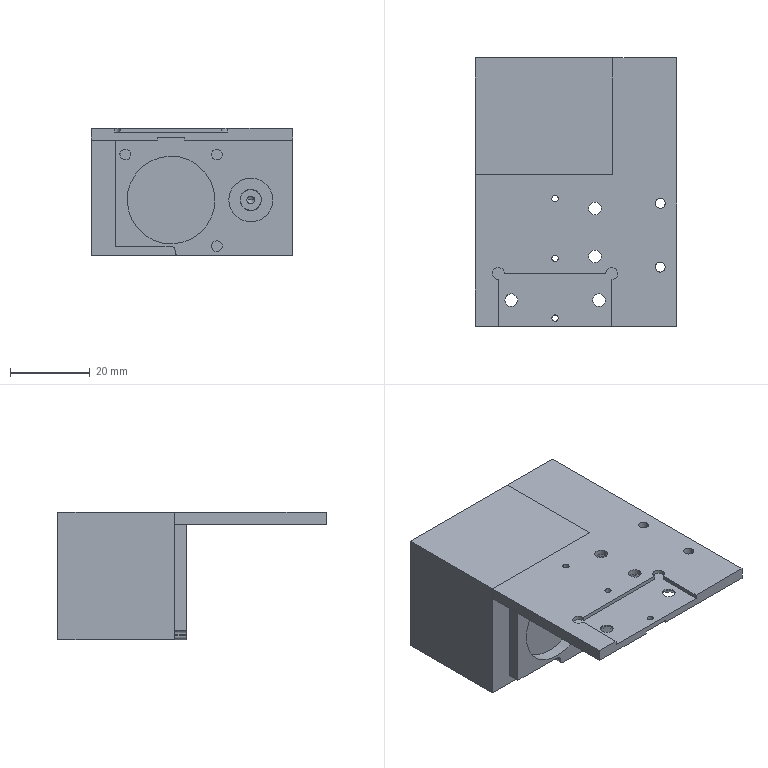NC program | NX | posted with a generic post | part box 50.5 x 67.3 x 32 mm
Whole program:
N10 G17 G21 G94 G90
(FLOOR_WALL_COPY , TOOL : D63)
N12 T01 M6
N14 G54
N16 G17 G0 G90 X68.15 Y-25.247 B0. C0. S6500 M3
N18 G43 Z30. H1
N20 Z5.
N22 G94 G1 Z2. F1500.
N24 X65.15
N26 X-65.15
N28 Y0.05
N30 X65.15
N32 X68.15
N34 Z5.
N36 G0 Z30.
N38 Y-25.247
N40 Z4.
N42 G1 Z1.
N44 X65.15
N46 X-65.15
N48 Y0.05
N50 X65.15
N52 X68.15
N54 Z4.
N56 G0 Z30.
N58 Y-25.247
N60 Z3.
N62 G1 Z0.
N64 X65.15
N66 X-65.15
N68 Y0.05
N70 X65.15
N72 X68.15
N74 Z3.
N76 G0 Z30.
N78 M5
(FLOOR_WALL_1_COPY_COPY_COPY , TOOL : D10)
N80 T10 M6
N82 G54
N84 G17 G0 G90 X-3.118 Y25.25 B0. C0. S9500 M3
N86 G43 Z30. H10
N88 Z-13.5
N90 G94 G1 Z-14.5 F1000.
N92 X-4.1 Y24.683
N94 G3 X-4.35 Y24.25 R0.5
N96 G1 X3.65 F1500.
N98 Y-25.25
N100 G3 X4.15 Y-26.116 R1.
N102 G1 X4.65 Y-26.405
N104 Z-13.5
N106 G0 Z30.
N108 X-3.118 Y25.25
N110 Z-28.
N112 G1 Z-29. F1000.
N114 X-4.1 Y24.683
N116 G3 X-4.35 Y24.25 R0.5
N118 G1 X3.65 F1500.
N120 Y-25.25
N122 G3 X4.15 Y-26.116 R1.
N124 G1 X4.65 Y-26.405
N126 Z-28.
N128 G0 Z30.
(PLANAR_MILL_COPY_1 , TOOL : D6A45)
N130 T07 M6
N132 G17 G43 G0 G90 X-27.098 Y-13.984 Z30. B0. C0. S9500 H7 M3
N134 Z2.
N136 G94 G1 Z-1. F1250.
N138 G3 X-27.455 Y-14.75 R1.
N140 X-25.65 Y-16.555 R1.805
N142 X-23.845 Y-14.75 R1.805
N144 X-25.65 Y-12.945 R1.805
N146 X-27.455 Y-14.75 R1.805
N148 X-27.098 Y-15.516 R1.
N150 G1 Z2.
N152 G0 Z30.
N154 X-22.484 Y-26.507
N156 Z2.
N158 G1 Z-1.
N160 G3 X-23.25 Y-26.15 R1.
N162 G1 X-33.65
N164 G2 X-34.55 Y-25.25 R0.9
N166 G1 Y-9.25
N168 G2 X-33.65 Y-8.35 R0.9
N170 G1 X-12.85
N172 G2 X-11.95 Y-9.25 R0.9
N174 G1 Y-25.25
N176 G2 X-12.85 Y-26.15 R0.9
N178 G1 X-23.25
N180 G3 X-24.016 Y-26.507 R1.
N182 G1 Z2.
N184 G0 Z30.
N186 X-16.002 Y-17.18
N188 Z2.
N190 G1 Z-1.
N192 G3 X-16.05 Y-17.6 R0.5
N194 X-15.7 Y-17.25 R0.35
N196 X-16.05 Y-16.9 R0.35
N198 X-16.4 Y-17.25 R0.35
N200 X-16.05 Y-17.6 R0.35
N202 X-16.098 Y-17.18 R0.5
N204 G1 Z2.
N206 G0 Z30.
N208 X-0.093 Y-9.734
N210 Z2.
N212 G1 Z-1.
N214 G3 X-0.45 Y-10.5 R1.
N216 G1 Y-25.25
N218 G2 X-1.35 Y-26.15 R0.9
N220 G1 X-4.35
N222 G2 X-5.25 Y-25.25 R0.9
N224 G1 Y4.25
N226 G2 X-4.35 Y5.15 R0.9
N228 G1 X-1.35
N230 G2 X-0.45 Y4.25 R0.9
N232 G1 Y-10.5
N234 G3 X-0.093 Y-11.266 R1.
N236 G1 Z2.
N238 G0 Z30.
N240 M5
N242 M2